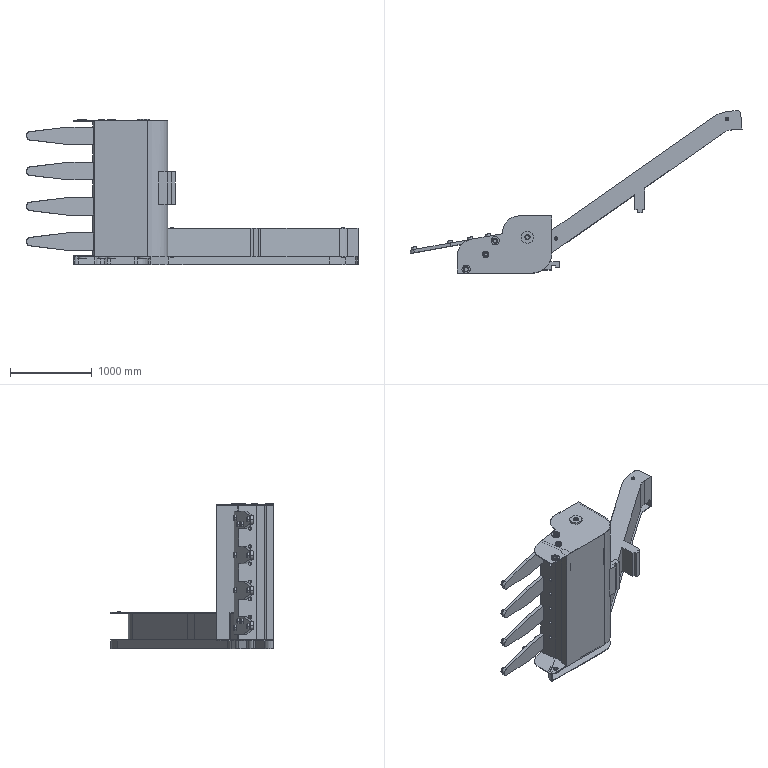Part | SolidWorks | 1 solid | 317 faces | box 4060 x 1991 x 1785 mm | volume 166702923 mm3 | cylinder 178 | plane 139 | commonest cylinder face diameters 40 x54 60 x28 100 x16 65 x14 20 x8 32 x8